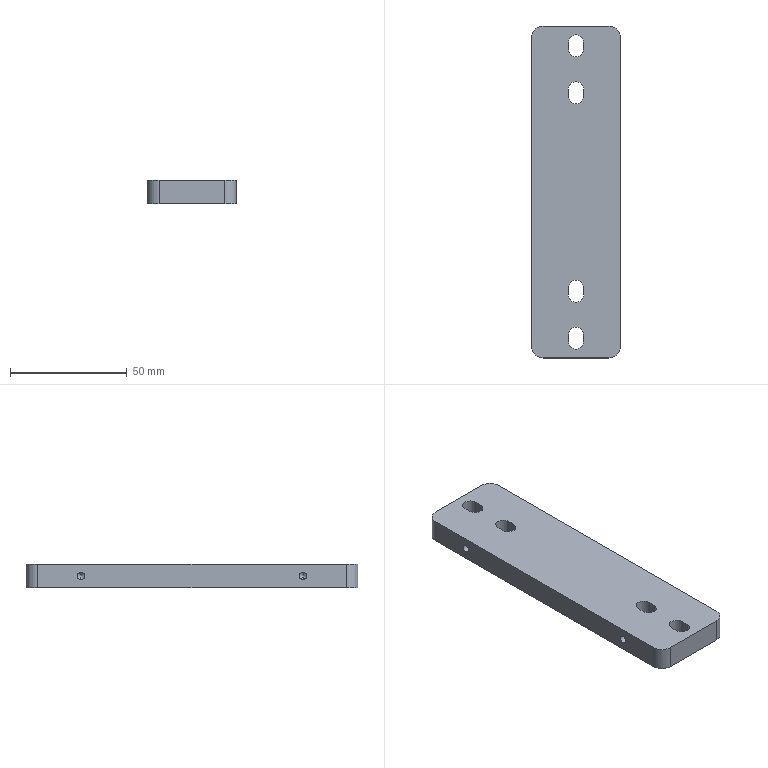Part | STEP file | 1 solid | 34 faces | box 38 x 142 x 10 mm | volume 51461 mm3 | cylinder 16 | plane 14 | cone 4 | commonest cylinder face diameters 6.5 x8 3.3 x4 10 x4